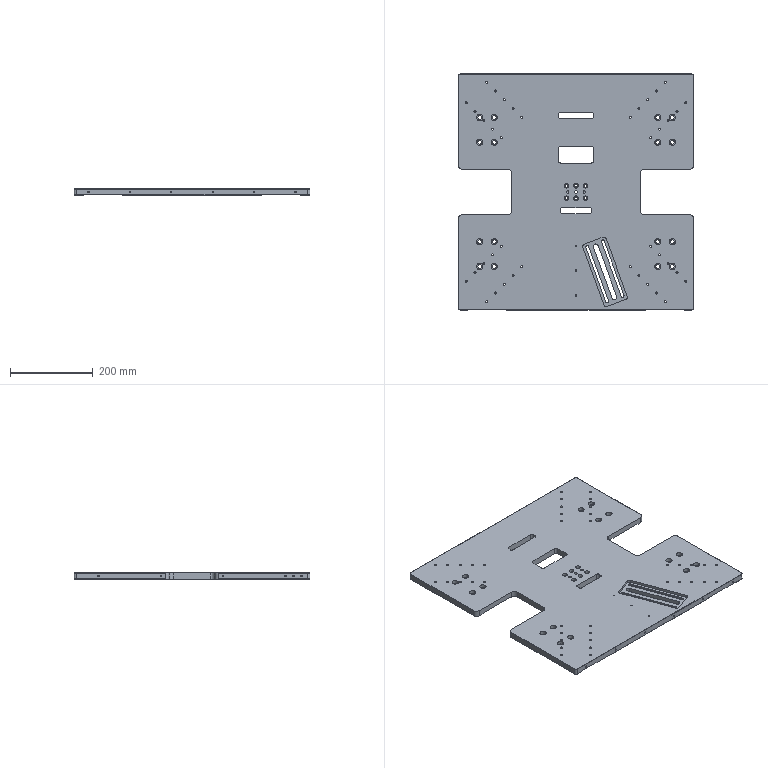Part | STEP file | 1 solid | 440 faces | box 570 x 570 x 15 mm | volume 4074607 mm3 | cylinder 276 | plane 104 | cone 60 | commonest cylinder face diameters 5 x80 9 x32 15 x32 3.3 x30 4.2 x24 10 x16